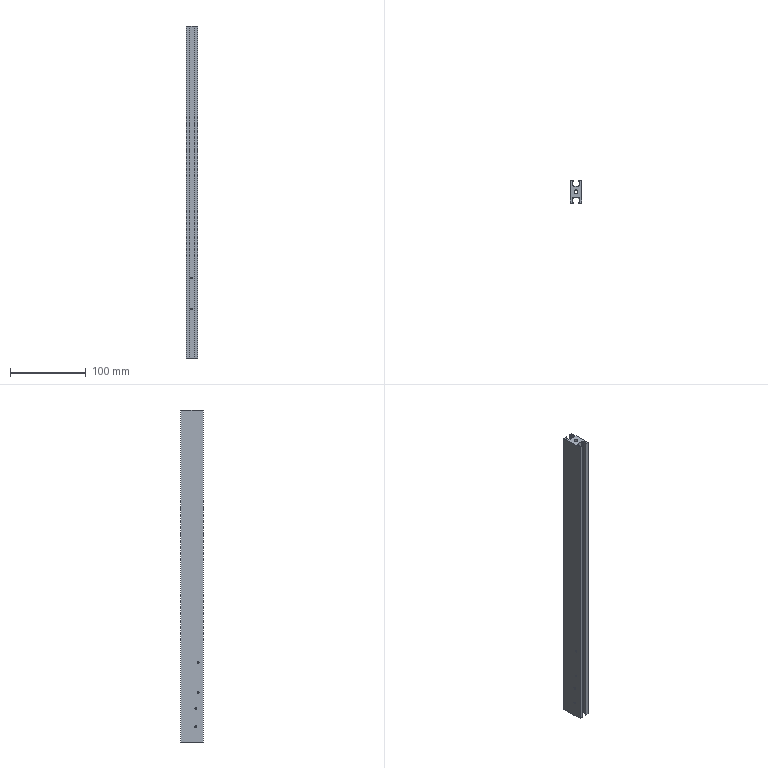Part | SolidWorks | features BaseBody 1 | 1 solid | 50 faces | box 15 x 30 x 438 mm | volume 123194 mm3 | plane 34 | cylinder 10 | cone 6 | commonest cylinder face diameters 2.5 x8 5 x2